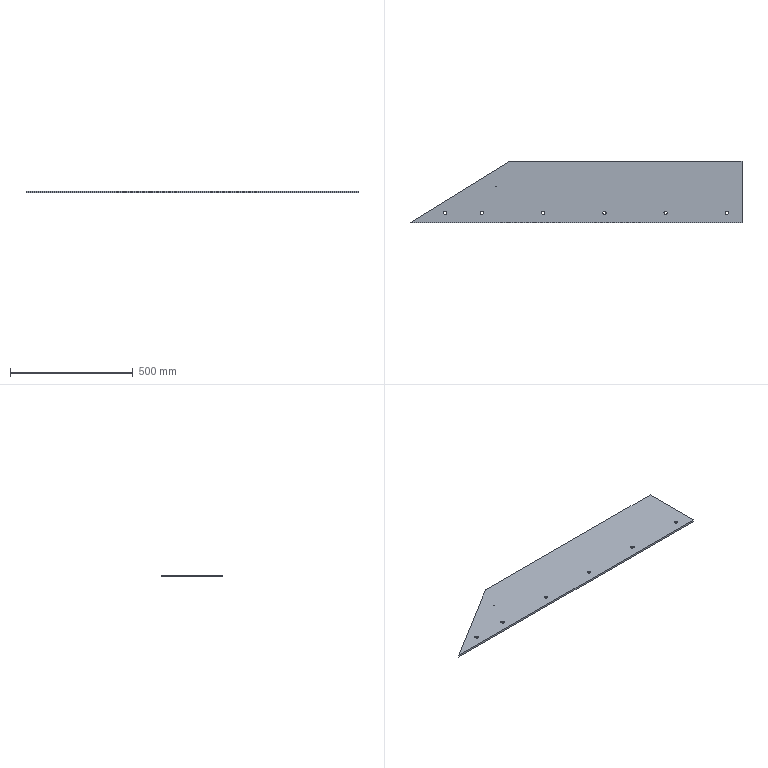Part | STEP file | Rubber plate 1_Default<As machined> | 1 solid | 20 faces | box 1355 x 250 x 8 mm | volume 2297597 mm3 | cylinder 14 | plane 6 | commonest cylinder face diameters 14 x12 1.5 x2